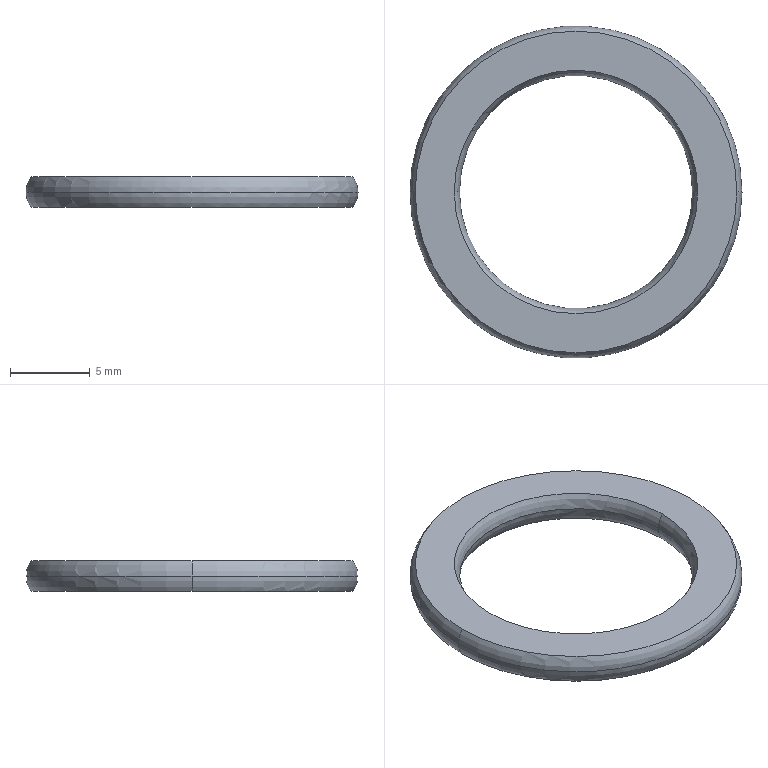Part | Creo | 1 solid | 10 faces | box 20.8 x 20.8 x 1.9 mm | volume 305.668 mm3 | torus 8 | plane 2
STEP:
#1=CARTESIAN_POINT('',(46.375,-75.,105.));
#2=VERTEX_POINT('',#1);
#3=CARTESIAN_POINT('',(61.625,-75.,105.));
#4=VERTEX_POINT('',#3);
#5=CARTESIAN_POINT('',(54.,-75.,105.));
#6=DIRECTION('',(0.,0.,1.));
#7=DIRECTION('',(-1.,0.,0.));
#8=AXIS2_PLACEMENT_3D('',#5,#6,#7);
#9=CIRCLE('',#8,7.625);
#10=EDGE_CURVE('',#2,#4,#9,.T.);
#11=ORIENTED_EDGE('',*,*,#10,.T.);
#12=CARTESIAN_POINT('',(61.3,-75.,105.95));
#13=VERTEX_POINT('',#12);
#14=CARTESIAN_POINT('',(62.85,-75.,105.95));
#15=DIRECTION('',(0.,-1.,0.));
#16=DIRECTION('',(-1.,0.,0.));
#17=AXIS2_PLACEMENT_3D('',#14,#15,#16);
#18=CIRCLE('',#17,1.55);
#19=EDGE_CURVE('',#13,#4,#18,.T.);
#20=ORIENTED_EDGE('',*,*,#19,.F.);
#21=CARTESIAN_POINT('',(46.7,-75.,105.95));
#22=VERTEX_POINT('',#21);
#23=CARTESIAN_POINT('',(54.,-75.,105.95));
#24=DIRECTION('',(0.,0.,1.));
#25=DIRECTION('',(-1.,0.,0.));
#26=AXIS2_PLACEMENT_3D('',#23,#24,#25);
#27=CIRCLE('',#26,7.3);
#28=EDGE_CURVE('',#22,#13,#27,.T.);
#29=ORIENTED_EDGE('',*,*,#28,.F.);
#30=CARTESIAN_POINT('',(45.15,-75.,105.95));
#31=DIRECTION('',(0.,1.,0.));
#32=DIRECTION('',(1.,0.,0.));
#33=AXIS2_PLACEMENT_3D('',#30,#31,#32);
#34=CIRCLE('',#33,1.55);
#35=EDGE_CURVE('',#22,#2,#34,.T.);
#36=ORIENTED_EDGE('',*,*,#35,.T.);
#37=EDGE_LOOP('',(#11,#20,#29,#36));
#38=FACE_OUTER_BOUND('',#37,.F.);
#39=CARTESIAN_POINT('',(54.,-75.,105.95));
#40=DIRECTION('',(0.,0.,1.));
#41=DIRECTION('',(-1.,0.,0.));
#42=AXIS2_PLACEMENT_3D('',#39,#40,#41);
#43=TOROIDAL_SURFACE('',#42,8.85,1.55);
#44=ADVANCED_FACE('',(#38),#43,.T.);
#45=CARTESIAN_POINT('',(64.075,-75.,105.));
#46=VERTEX_POINT('',#45);
#47=CARTESIAN_POINT('',(43.925,-75.,105.));
#48=VERTEX_POINT('',#47);
#49=CARTESIAN_POINT('',(54.,-75.,105.));
#50=DIRECTION('',(0.,0.,-1.));
#51=DIRECTION('',(1.,0.,0.));
#52=AXIS2_PLACEMENT_3D('',#49,#50,#51);
#53=CIRCLE('',#52,10.075);
#54=EDGE_CURVE('',#46,#48,#53,.T.);
#55=ORIENTED_EDGE('',*,*,#54,.F.);
#56=CARTESIAN_POINT('',(54.,-75.,105.));
#57=DIRECTION('',(0.,0.,-1.));
#58=DIRECTION('',(-1.,0.,0.));
#59=AXIS2_PLACEMENT_3D('',#56,#57,#58);
#60=CIRCLE('',#59,10.075);
#61=EDGE_CURVE('',#48,#46,#60,.T.);
#62=ORIENTED_EDGE('',*,*,#61,.F.);
#63=EDGE_LOOP('',(#55,#62));
#64=FACE_OUTER_BOUND('',#63,.F.);
#65=CARTESIAN_POINT('',(54.,-75.,105.));
#66=DIRECTION('',(0.,0.,1.));
#67=DIRECTION('',(1.,0.,0.));
#68=AXIS2_PLACEMENT_3D('',#65,#66,#67);
#69=CIRCLE('',#68,7.625);
#70=EDGE_CURVE('',#4,#2,#69,.T.);
#71=ORIENTED_EDGE('',*,*,#70,.F.);
#72=ORIENTED_EDGE('',*,*,#10,.F.);
#73=EDGE_LOOP('',(#71,#72));
#74=FACE_BOUND('',#73,.F.);
#75=CARTESIAN_POINT('',(54.,-64.925,105.));
#76=DIRECTION('',(0.,0.,-1.));
#77=DIRECTION('',(1.,0.,0.));
#78=AXIS2_PLACEMENT_3D('',#75,#76,#77);
#79=PLANE('',#78);
#80=ADVANCED_FACE('',(#64,#74),#79,.T.);
#81=ORIENTED_EDGE('',*,*,#70,.T.);
#82=ORIENTED_EDGE('',*,*,#35,.F.);
#83=CARTESIAN_POINT('',(54.,-75.,105.95));
#84=DIRECTION('',(0.,0.,1.));
#85=DIRECTION('',(1.,0.,0.));
#86=AXIS2_PLACEMENT_3D('',#83,#84,#85);
#87=CIRCLE('',#86,7.3);
#88=EDGE_CURVE('',#13,#22,#87,.T.);
#89=ORIENTED_EDGE('',*,*,#88,.F.);
#90=ORIENTED_EDGE('',*,*,#19,.T.);
#91=EDGE_LOOP('',(#81,#82,#89,#90));
#92=FACE_OUTER_BOUND('',#91,.F.);
#93=CARTESIAN_POINT('',(54.,-75.,105.95));
#94=DIRECTION('',(0.,0.,1.));
#95=DIRECTION('',(-1.,0.,0.));
#96=AXIS2_PLACEMENT_3D('',#93,#94,#95);
#97=TOROIDAL_SURFACE('',#96,8.85,1.55);
#98=ADVANCED_FACE('',(#92),#97,.T.);
#99=CARTESIAN_POINT('',(46.375,-75.,106.9));
#100=VERTEX_POINT('',#99);
#101=CARTESIAN_POINT('',(61.625,-75.,106.9));
#102=VERTEX_POINT('',#101);
#103=CARTESIAN_POINT('',(54.,-75.,106.9));
#104=DIRECTION('',(0.,0.,-1.));
#105=DIRECTION('',(-1.,0.,0.));
#106=AXIS2_PLACEMENT_3D('',#103,#104,#105);
#107=CIRCLE('',#106,7.625);
#108=EDGE_CURVE('',#100,#102,#107,.T.);
#109=ORIENTED_EDGE('',*,*,#108,.T.);
#110=CARTESIAN_POINT('',(62.85,-75.,105.95));
#111=DIRECTION('',(0.,-1.,0.));
#112=DIRECTION('',(-0.7902,0.,0.6129));
#113=AXIS2_PLACEMENT_3D('',#110,#111,#112);
#114=CIRCLE('',#113,1.55);
#115=EDGE_CURVE('',#102,#13,#114,.T.);
#116=ORIENTED_EDGE('',*,*,#115,.T.);
#117=ORIENTED_EDGE('',*,*,#88,.T.);
#118=CARTESIAN_POINT('',(45.15,-75.,105.95));
#119=DIRECTION('',(0.,1.,0.));
#120=DIRECTION('',(0.7902,0.,0.6129));
#121=AXIS2_PLACEMENT_3D('',#118,#119,#120);
#122=CIRCLE('',#121,1.55);
#123=EDGE_CURVE('',#100,#22,#122,.T.);
#124=ORIENTED_EDGE('',*,*,#123,.F.);
#125=EDGE_LOOP('',(#109,#116,#117,#124));
#126=FACE_OUTER_BOUND('',#125,.F.);
#127=CARTESIAN_POINT('',(54.,-75.,105.95));
#128=DIRECTION('',(0.,0.,1.));
#129=DIRECTION('',(-1.,0.,0.));
#130=AXIS2_PLACEMENT_3D('',#127,#128,#129);
#131=TOROIDAL_SURFACE('',#130,8.85,1.55);
#132=ADVANCED_FACE('',(#126),#131,.T.);
#133=CARTESIAN_POINT('',(64.075,-75.,106.9));
#134=VERTEX_POINT('',#133);
#135=CARTESIAN_POINT('',(43.925,-75.,106.9));
#136=VERTEX_POINT('',#135);
#137=CARTESIAN_POINT('',(54.,-75.,106.9));
#138=DIRECTION('',(0.,0.,1.));
#139=DIRECTION('',(1.,0.,0.));
#140=AXIS2_PLACEMENT_3D('',#137,#138,#139);
#141=CIRCLE('',#140,10.075);
#142=EDGE_CURVE('',#134,#136,#141,.T.);
#143=ORIENTED_EDGE('',*,*,#142,.F.);
#144=CARTESIAN_POINT('',(54.,-75.,106.9));
#145=DIRECTION('',(0.,0.,1.));
#146=DIRECTION('',(-1.,0.,0.));
#147=AXIS2_PLACEMENT_3D('',#144,#145,#146);
#148=CIRCLE('',#147,10.075);
#149=EDGE_CURVE('',#136,#134,#148,.T.);
#150=ORIENTED_EDGE('',*,*,#149,.F.);
#151=EDGE_LOOP('',(#143,#150));
#152=FACE_OUTER_BOUND('',#151,.F.);
#153=CARTESIAN_POINT('',(54.,-75.,106.9));
#154=DIRECTION('',(0.,0.,-1.));
#155=DIRECTION('',(1.,0.,0.));
#156=AXIS2_PLACEMENT_3D('',#153,#154,#155);
#157=CIRCLE('',#156,7.625);
#158=EDGE_CURVE('',#102,#100,#157,.T.);
#159=ORIENTED_EDGE('',*,*,#158,.F.);
#160=ORIENTED_EDGE('',*,*,#108,.F.);
#161=EDGE_LOOP('',(#159,#160));
#162=FACE_BOUND('',#161,.F.);
#163=CARTESIAN_POINT('',(54.,-67.375,106.9));
#164=DIRECTION('',(0.,0.,1.));
#165=DIRECTION('',(-1.,0.,0.));
#166=AXIS2_PLACEMENT_3D('',#163,#164,#165);
#167=PLANE('',#166);
#168=ADVANCED_FACE('',(#152,#162),#167,.T.);
#169=ORIENTED_EDGE('',*,*,#142,.T.);
#170=CARTESIAN_POINT('',(43.6,-75.,105.95));
#171=VERTEX_POINT('',#170);
#172=CARTESIAN_POINT('',(45.15,-75.,105.95));
#173=DIRECTION('',(0.,1.,0.));
#174=DIRECTION('',(-1.,0.,0.));
#175=AXIS2_PLACEMENT_3D('',#172,#173,#174);
#176=CIRCLE('',#175,1.55);
#177=EDGE_CURVE('',#171,#136,#176,.T.);
#178=ORIENTED_EDGE('',*,*,#177,.F.);
#179=CARTESIAN_POINT('',(64.4,-75.,105.95));
#180=VERTEX_POINT('',#179);
#181=CARTESIAN_POINT('',(54.,-75.,105.95));
#182=DIRECTION('',(0.,0.,1.));
#183=DIRECTION('',(1.,0.,0.));
#184=AXIS2_PLACEMENT_3D('',#181,#182,#183);
#185=CIRCLE('',#184,10.4);
#186=EDGE_CURVE('',#180,#171,#185,.T.);
#187=ORIENTED_EDGE('',*,*,#186,.F.);
#188=CARTESIAN_POINT('',(62.85,-75.,105.95));
#189=DIRECTION('',(0.,-1.,0.));
#190=DIRECTION('',(1.,0.,0.));
#191=AXIS2_PLACEMENT_3D('',#188,#189,#190);
#192=CIRCLE('',#191,1.55);
#193=EDGE_CURVE('',#180,#134,#192,.T.);
#194=ORIENTED_EDGE('',*,*,#193,.T.);
#195=EDGE_LOOP('',(#169,#178,#187,#194));
#196=FACE_OUTER_BOUND('',#195,.F.);
#197=CARTESIAN_POINT('',(54.,-75.,105.95));
#198=DIRECTION('',(0.,0.,1.));
#199=DIRECTION('',(-1.,0.,0.));
#200=AXIS2_PLACEMENT_3D('',#197,#198,#199);
#201=TOROIDAL_SURFACE('',#200,8.85,1.55);
#202=ADVANCED_FACE('',(#196),#201,.T.);
#203=ORIENTED_EDGE('',*,*,#149,.T.);
#204=ORIENTED_EDGE('',*,*,#193,.F.);
#205=CARTESIAN_POINT('',(54.,-75.,105.95));
#206=DIRECTION('',(0.,0.,1.));
#207=DIRECTION('',(-1.,0.,0.));
#208=AXIS2_PLACEMENT_3D('',#205,#206,#207);
#209=CIRCLE('',#208,10.4);
#210=EDGE_CURVE('',#171,#180,#209,.T.);
#211=ORIENTED_EDGE('',*,*,#210,.F.);
#212=ORIENTED_EDGE('',*,*,#177,.T.);
#213=EDGE_LOOP('',(#203,#204,#211,#212));
#214=FACE_OUTER_BOUND('',#213,.F.);
#215=CARTESIAN_POINT('',(54.,-75.,105.95));
#216=DIRECTION('',(0.,0.,1.));
#217=DIRECTION('',(-1.,0.,0.));
#218=AXIS2_PLACEMENT_3D('',#215,#216,#217);
#219=TOROIDAL_SURFACE('',#218,8.85,1.55);
#220=ADVANCED_FACE('',(#214),#219,.T.);
#221=ORIENTED_EDGE('',*,*,#54,.T.);
#222=CARTESIAN_POINT('',(45.15,-75.,105.95));
#223=DIRECTION('',(0.,1.,0.));
#224=DIRECTION('',(-0.7902,0.,-0.6129));
#225=AXIS2_PLACEMENT_3D('',#222,#223,#224);
#226=CIRCLE('',#225,1.55);
#227=EDGE_CURVE('',#48,#171,#226,.T.);
#228=ORIENTED_EDGE('',*,*,#227,.T.);
#229=ORIENTED_EDGE('',*,*,#210,.T.);
#230=CARTESIAN_POINT('',(62.85,-75.,105.95));
#231=DIRECTION('',(0.,-1.,0.));
#232=DIRECTION('',(0.7902,0.,-0.6129));
#233=AXIS2_PLACEMENT_3D('',#230,#231,#232);
#234=CIRCLE('',#233,1.55);
#235=EDGE_CURVE('',#46,#180,#234,.T.);
#236=ORIENTED_EDGE('',*,*,#235,.F.);
#237=EDGE_LOOP('',(#221,#228,#229,#236));
#238=FACE_OUTER_BOUND('',#237,.F.);
#239=CARTESIAN_POINT('',(54.,-75.,105.95));
#240=DIRECTION('',(0.,0.,1.));
#241=DIRECTION('',(-1.,0.,0.));
#242=AXIS2_PLACEMENT_3D('',#239,#240,#241);
#243=TOROIDAL_SURFACE('',#242,8.85,1.55);
#244=ADVANCED_FACE('',(#238),#243,.T.);
#245=ORIENTED_EDGE('',*,*,#61,.T.);
#246=ORIENTED_EDGE('',*,*,#235,.T.);
#247=ORIENTED_EDGE('',*,*,#186,.T.);
#248=ORIENTED_EDGE('',*,*,#227,.F.);
#249=EDGE_LOOP('',(#245,#246,#247,#248));
#250=FACE_OUTER_BOUND('',#249,.F.);
#251=CARTESIAN_POINT('',(54.,-75.,105.95));
#252=DIRECTION('',(0.,0.,1.));
#253=DIRECTION('',(-1.,0.,0.));
#254=AXIS2_PLACEMENT_3D('',#251,#252,#253);
#255=TOROIDAL_SURFACE('',#254,8.85,1.55);
#256=ADVANCED_FACE('',(#250),#255,.T.);
#257=ORIENTED_EDGE('',*,*,#158,.T.);
#258=ORIENTED_EDGE('',*,*,#123,.T.);
#259=ORIENTED_EDGE('',*,*,#28,.T.);
#260=ORIENTED_EDGE('',*,*,#115,.F.);
#261=EDGE_LOOP('',(#257,#258,#259,#260));
#262=FACE_OUTER_BOUND('',#261,.F.);
#263=CARTESIAN_POINT('',(54.,-75.,105.95));
#264=DIRECTION('',(0.,0.,1.));
#265=DIRECTION('',(-1.,0.,0.));
#266=AXIS2_PLACEMENT_3D('',#263,#264,#265);
#267=TOROIDAL_SURFACE('',#266,8.85,1.55);
#268=ADVANCED_FACE('',(#262),#267,.T.);
#269=CLOSED_SHELL('',(#44,#80,#98,#132,#168,#202,#220,#244,#256,#268));
#270=MANIFOLD_SOLID_BREP('',#269);
#271=(LENGTH_UNIT()NAMED_UNIT(*)SI_UNIT(.MILLI.,.METRE.));
#272=UNCERTAINTY_MEASURE_WITH_UNIT(LENGTH_MEASURE(0.002948),#271,'','');
#273=(NAMED_UNIT(*)PLANE_ANGLE_UNIT()SI_UNIT($,.RADIAN.));
#274=PLANE_ANGLE_MEASURE_WITH_UNIT(PLANE_ANGLE_MEASURE(0.01745),#273);
#275=(CONVERSION_BASED_UNIT('DEGREE',#274)NAMED_UNIT(*)PLANE_ANGLE_UNIT());
#276=(NAMED_UNIT(*)SI_UNIT($,.STERADIAN.)SOLID_ANGLE_UNIT());
#277=(GEOMETRIC_REPRESENTATION_CONTEXT(3)GLOBAL_UNCERTAINTY_ASSIGNED_CONTEXT((#272))GLOBAL_UNIT_ASSIGNED_CONTEXT((#271,#275,#276))REPRESENTATION_CONTEXT('',''));
#278=ADVANCED_BREP_SHAPE_REPRESENTATION('',(#270),#277);